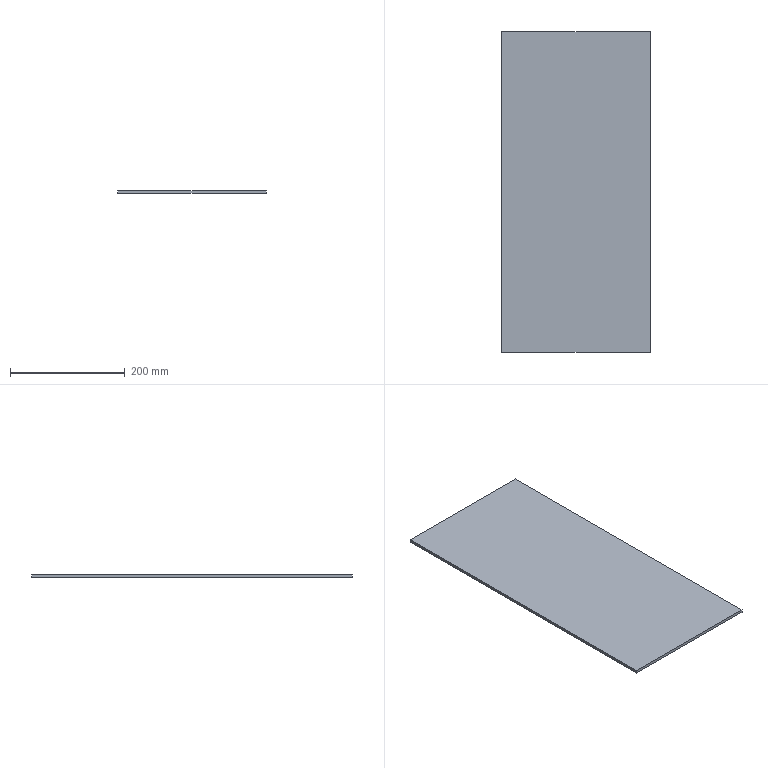Part | SolidWorks | features BaseBody 1 | 1 solid | 6 faces | box 260 x 560 x 5 mm | volume 728000 mm3 | plane 6
STEP:
#1=CARTESIAN_POINT('',(-600.,600.,-395.));
#2=VERTEX_POINT('',#1);
#3=CARTESIAN_POINT('',(-600.,40.,-395.));
#4=VERTEX_POINT('',#3);
#5=CARTESIAN_POINT('',(-600.,600.,-395.));
#6=DIRECTION('',(0.,-1.,0.));
#7=VECTOR('',#6,1000.);
#8=LINE('',#5,#7);
#9=EDGE_CURVE('',#2,#4,#8,.T.);
#10=ORIENTED_EDGE('',*,*,#9,.F.);
#11=CARTESIAN_POINT('',(-860.,600.,-395.));
#12=VERTEX_POINT('',#11);
#13=CARTESIAN_POINT('',(-860.,600.,-395.));
#14=DIRECTION('',(1.,0.,0.));
#15=VECTOR('',#14,1000.);
#16=LINE('',#13,#15);
#17=EDGE_CURVE('',#12,#2,#16,.T.);
#18=ORIENTED_EDGE('',*,*,#17,.F.);
#19=CARTESIAN_POINT('',(-860.,40.,-395.));
#20=VERTEX_POINT('',#19);
#21=CARTESIAN_POINT('',(-860.,40.,-395.));
#22=DIRECTION('',(0.,1.,0.));
#23=VECTOR('',#22,1000.);
#24=LINE('',#21,#23);
#25=EDGE_CURVE('',#20,#12,#24,.T.);
#26=ORIENTED_EDGE('',*,*,#25,.F.);
#27=CARTESIAN_POINT('',(-600.,40.,-395.));
#28=DIRECTION('',(-1.,0.,0.));
#29=VECTOR('',#28,1000.);
#30=LINE('',#27,#29);
#31=EDGE_CURVE('',#4,#20,#30,.T.);
#32=ORIENTED_EDGE('',*,*,#31,.F.);
#33=EDGE_LOOP('',(#10,#18,#26,#32));
#34=FACE_OUTER_BOUND('',#33,.T.);
#35=CARTESIAN_POINT('',(-730.,320.,-395.));
#36=DIRECTION('',(0.,0.,1.));
#37=DIRECTION('',(1.,0.,0.));
#38=AXIS2_PLACEMENT_3D('',#35,#36,#37);
#39=PLANE('',#38);
#40=ADVANCED_FACE('',(#34),#39,.T.);
#41=CARTESIAN_POINT('',(-600.,40.,-400.));
#42=VERTEX_POINT('',#41);
#43=CARTESIAN_POINT('',(-600.,600.,-400.));
#44=VERTEX_POINT('',#43);
#45=CARTESIAN_POINT('',(-600.,40.,-400.));
#46=DIRECTION('',(0.,1.,0.));
#47=VECTOR('',#46,1000.);
#48=LINE('',#45,#47);
#49=EDGE_CURVE('',#42,#44,#48,.T.);
#50=ORIENTED_EDGE('',*,*,#49,.F.);
#51=CARTESIAN_POINT('',(-860.,40.,-400.));
#52=VERTEX_POINT('',#51);
#53=CARTESIAN_POINT('',(-860.,40.,-400.));
#54=DIRECTION('',(1.,0.,0.));
#55=VECTOR('',#54,1000.);
#56=LINE('',#53,#55);
#57=EDGE_CURVE('',#52,#42,#56,.T.);
#58=ORIENTED_EDGE('',*,*,#57,.F.);
#59=CARTESIAN_POINT('',(-860.,600.,-400.));
#60=VERTEX_POINT('',#59);
#61=CARTESIAN_POINT('',(-860.,600.,-400.));
#62=DIRECTION('',(0.,-1.,0.));
#63=VECTOR('',#62,1000.);
#64=LINE('',#61,#63);
#65=EDGE_CURVE('',#60,#52,#64,.T.);
#66=ORIENTED_EDGE('',*,*,#65,.F.);
#67=CARTESIAN_POINT('',(-600.,600.,-400.));
#68=DIRECTION('',(-1.,0.,0.));
#69=VECTOR('',#68,1000.);
#70=LINE('',#67,#69);
#71=EDGE_CURVE('',#44,#60,#70,.T.);
#72=ORIENTED_EDGE('',*,*,#71,.F.);
#73=EDGE_LOOP('',(#50,#58,#66,#72));
#74=FACE_OUTER_BOUND('',#73,.T.);
#75=CARTESIAN_POINT('',(-730.,320.,-400.));
#76=DIRECTION('',(0.,0.,-1.));
#77=DIRECTION('',(0.,-1.,0.));
#78=AXIS2_PLACEMENT_3D('',#75,#76,#77);
#79=PLANE('',#78);
#80=ADVANCED_FACE('',(#74),#79,.T.);
#81=ORIENTED_EDGE('',*,*,#49,.T.);
#82=CARTESIAN_POINT('',(-600.,600.,-395.));
#83=DIRECTION('',(0.,0.,-1.));
#84=VECTOR('',#83,1000.);
#85=LINE('',#82,#84);
#86=EDGE_CURVE('',#2,#44,#85,.T.);
#87=ORIENTED_EDGE('',*,*,#86,.F.);
#88=ORIENTED_EDGE('',*,*,#9,.T.);
#89=CARTESIAN_POINT('',(-600.,40.,-400.));
#90=DIRECTION('',(0.,0.,1.));
#91=VECTOR('',#90,1000.);
#92=LINE('',#89,#91);
#93=EDGE_CURVE('',#42,#4,#92,.T.);
#94=ORIENTED_EDGE('',*,*,#93,.F.);
#95=EDGE_LOOP('',(#81,#87,#88,#94));
#96=FACE_OUTER_BOUND('',#95,.T.);
#97=CARTESIAN_POINT('',(-600.,40.,-400.));
#98=DIRECTION('',(1.,0.,0.));
#99=DIRECTION('',(0.,1.,0.));
#100=AXIS2_PLACEMENT_3D('',#97,#98,#99);
#101=PLANE('',#100);
#102=ADVANCED_FACE('',(#96),#101,.T.);
#103=ORIENTED_EDGE('',*,*,#71,.T.);
#104=CARTESIAN_POINT('',(-860.,600.,-395.));
#105=DIRECTION('',(0.,0.,-1.));
#106=VECTOR('',#105,1000.);
#107=LINE('',#104,#106);
#108=EDGE_CURVE('',#12,#60,#107,.T.);
#109=ORIENTED_EDGE('',*,*,#108,.F.);
#110=ORIENTED_EDGE('',*,*,#17,.T.);
#111=ORIENTED_EDGE('',*,*,#86,.T.);
#112=EDGE_LOOP('',(#103,#109,#110,#111));
#113=FACE_OUTER_BOUND('',#112,.T.);
#114=CARTESIAN_POINT('',(-600.,600.,-400.));
#115=DIRECTION('',(0.,1.,0.));
#116=DIRECTION('',(1.,0.,0.));
#117=AXIS2_PLACEMENT_3D('',#114,#115,#116);
#118=PLANE('',#117);
#119=ADVANCED_FACE('',(#113),#118,.T.);
#120=ORIENTED_EDGE('',*,*,#65,.T.);
#121=CARTESIAN_POINT('',(-860.,40.,-395.));
#122=DIRECTION('',(0.,0.,-1.));
#123=VECTOR('',#122,1000.);
#124=LINE('',#121,#123);
#125=EDGE_CURVE('',#20,#52,#124,.T.);
#126=ORIENTED_EDGE('',*,*,#125,.F.);
#127=ORIENTED_EDGE('',*,*,#25,.T.);
#128=ORIENTED_EDGE('',*,*,#108,.T.);
#129=EDGE_LOOP('',(#120,#126,#127,#128));
#130=FACE_OUTER_BOUND('',#129,.T.);
#131=CARTESIAN_POINT('',(-860.,600.,-400.));
#132=DIRECTION('',(-1.,0.,0.));
#133=DIRECTION('',(0.,0.,1.));
#134=AXIS2_PLACEMENT_3D('',#131,#132,#133);
#135=PLANE('',#134);
#136=ADVANCED_FACE('',(#130),#135,.T.);
#137=ORIENTED_EDGE('',*,*,#57,.T.);
#138=ORIENTED_EDGE('',*,*,#93,.T.);
#139=ORIENTED_EDGE('',*,*,#31,.T.);
#140=ORIENTED_EDGE('',*,*,#125,.T.);
#141=EDGE_LOOP('',(#137,#138,#139,#140));
#142=FACE_OUTER_BOUND('',#141,.T.);
#143=CARTESIAN_POINT('',(-860.,40.,-400.));
#144=DIRECTION('',(0.,-1.,0.));
#145=DIRECTION('',(0.,0.,-1.));
#146=AXIS2_PLACEMENT_3D('',#143,#144,#145);
#147=PLANE('',#146);
#148=ADVANCED_FACE('',(#142),#147,.T.);
#149=CLOSED_SHELL('',(#40,#80,#102,#119,#136,#148));
#150=MANIFOLD_SOLID_BREP('',#149);
#151=CARTESIAN_POINT('',(0.,0.,0.));
#152=DIRECTION('',(0.,0.,1.));
#153=DIRECTION('',(1.,0.,0.));
#154=AXIS2_PLACEMENT_3D('',#151,#152,#153);
#155=(LENGTH_UNIT()NAMED_UNIT(*)SI_UNIT(.MILLI.,.METRE.));
#156=UNCERTAINTY_MEASURE_WITH_UNIT(LENGTH_MEASURE(0.00001),#155,'','');
#157=(NAMED_UNIT(*)PLANE_ANGLE_UNIT()SI_UNIT($,.RADIAN.));
#158=(NAMED_UNIT(*)SI_UNIT($,.STERADIAN.)SOLID_ANGLE_UNIT());
#159=(GEOMETRIC_REPRESENTATION_CONTEXT(3)GLOBAL_UNCERTAINTY_ASSIGNED_CONTEXT((#156))GLOBAL_UNIT_ASSIGNED_CONTEXT((#155,#157,#158))REPRESENTATION_CONTEXT('',''));
#160=ADVANCED_BREP_SHAPE_REPRESENTATION('',(#150,#154),#159);